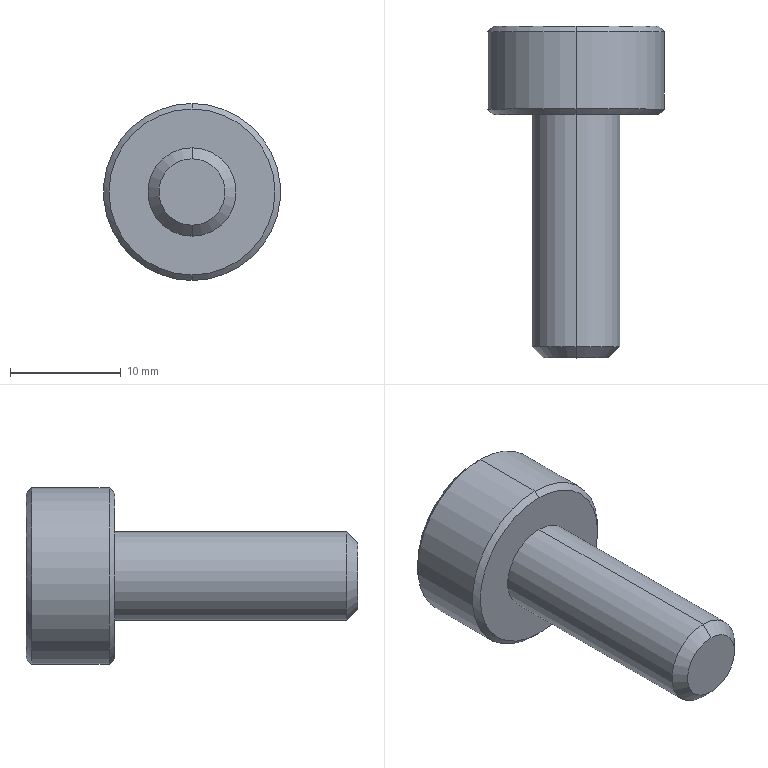Part | STEP file | Guide wheel mechanism revised.sldasm-Part-320 | 1 solid | 20 faces | box 16 x 30 x 16 mm | volume 2413 mm3 | plane 10 | cone 6 | cylinder 4 | commonest cylinder face diameters 8 x2 16 x2
STEP:
#1=CARTESIAN_POINT('',(0.,0.,-3.));
#2=VERTEX_POINT('',#1);
#3=CARTESIAN_POINT('',(0.,0.,3.));
#4=VERTEX_POINT('',#3);
#5=CARTESIAN_POINT('',(0.,0.,0.));
#6=DIRECTION('',(0.,-1.,0.));
#7=DIRECTION('',(0.,0.,-1.));
#8=AXIS2_PLACEMENT_3D('',#5,#6,#7);
#9=CIRCLE('',#8,3.);
#10=EDGE_CURVE('',#2,#4,#9,.T.);
#11=ORIENTED_EDGE('',*,*,#10,.F.);
#12=CARTESIAN_POINT('',(0.,1.,-4.));
#13=VERTEX_POINT('',#12);
#14=CARTESIAN_POINT('',(0.,0.,-3.));
#15=DIRECTION('',(0.,0.7071,-0.7071));
#16=VECTOR('',#15,1000.);
#17=LINE('',#14,#16);
#18=EDGE_CURVE('',#2,#13,#17,.T.);
#19=ORIENTED_EDGE('',*,*,#18,.T.);
#20=CARTESIAN_POINT('',(0.,1.,4.));
#21=VERTEX_POINT('',#20);
#22=CARTESIAN_POINT('',(0.,1.,0.));
#23=DIRECTION('',(0.,1.,0.));
#24=DIRECTION('',(0.,0.,-1.));
#25=AXIS2_PLACEMENT_3D('',#22,#23,#24);
#26=CIRCLE('',#25,4.);
#27=EDGE_CURVE('',#21,#13,#26,.T.);
#28=ORIENTED_EDGE('',*,*,#27,.F.);
#29=CARTESIAN_POINT('',(0.,0.,3.));
#30=DIRECTION('',(0.,0.7071,0.7071));
#31=VECTOR('',#30,1000.);
#32=LINE('',#29,#31);
#33=EDGE_CURVE('',#4,#21,#32,.T.);
#34=ORIENTED_EDGE('',*,*,#33,.F.);
#35=EDGE_LOOP('',(#11,#19,#28,#34));
#36=FACE_OUTER_BOUND('',#35,.T.);
#37=CARTESIAN_POINT('',(0.,0.,0.));
#38=DIRECTION('',(0.,1.,0.));
#39=DIRECTION('',(0.,0.,1.));
#40=AXIS2_PLACEMENT_3D('',#37,#38,#39);
#41=CONICAL_SURFACE('',#40,3.,0.7854);
#42=ADVANCED_FACE('',(#36),#41,.T.);
#43=CARTESIAN_POINT('',(0.,22.,-7.5));
#44=VERTEX_POINT('',#43);
#45=CARTESIAN_POINT('',(0.,22.,7.5));
#46=VERTEX_POINT('',#45);
#47=CARTESIAN_POINT('',(0.,22.,0.));
#48=DIRECTION('',(0.,-1.,0.));
#49=DIRECTION('',(0.,0.,-1.));
#50=AXIS2_PLACEMENT_3D('',#47,#48,#49);
#51=CIRCLE('',#50,7.5);
#52=EDGE_CURVE('',#44,#46,#51,.T.);
#53=ORIENTED_EDGE('',*,*,#52,.F.);
#54=CARTESIAN_POINT('',(0.,22.5,-8.));
#55=VERTEX_POINT('',#54);
#56=CARTESIAN_POINT('',(0.,22.,-7.5));
#57=DIRECTION('',(0.,0.7071,-0.7071));
#58=VECTOR('',#57,1000.);
#59=LINE('',#56,#58);
#60=EDGE_CURVE('',#44,#55,#59,.T.);
#61=ORIENTED_EDGE('',*,*,#60,.T.);
#62=CARTESIAN_POINT('',(0.,22.5,8.));
#63=VERTEX_POINT('',#62);
#64=CARTESIAN_POINT('',(0.,22.5,0.));
#65=DIRECTION('',(0.,1.,0.));
#66=DIRECTION('',(0.,0.,-1.));
#67=AXIS2_PLACEMENT_3D('',#64,#65,#66);
#68=CIRCLE('',#67,8.);
#69=EDGE_CURVE('',#63,#55,#68,.T.);
#70=ORIENTED_EDGE('',*,*,#69,.F.);
#71=CARTESIAN_POINT('',(0.,22.,7.5));
#72=DIRECTION('',(0.,0.7071,0.7071));
#73=VECTOR('',#72,1000.);
#74=LINE('',#71,#73);
#75=EDGE_CURVE('',#46,#63,#74,.T.);
#76=ORIENTED_EDGE('',*,*,#75,.F.);
#77=EDGE_LOOP('',(#53,#61,#70,#76));
#78=FACE_OUTER_BOUND('',#77,.T.);
#79=CARTESIAN_POINT('',(0.,22.,0.));
#80=DIRECTION('',(0.,1.,0.));
#81=DIRECTION('',(0.,0.,1.));
#82=AXIS2_PLACEMENT_3D('',#79,#80,#81);
#83=CONICAL_SURFACE('',#82,7.5,0.7854);
#84=ADVANCED_FACE('',(#78),#83,.T.);
#85=CARTESIAN_POINT('',(0.,30.,7.5));
#86=VERTEX_POINT('',#85);
#87=CARTESIAN_POINT('',(0.,30.,-7.5));
#88=VERTEX_POINT('',#87);
#89=CARTESIAN_POINT('',(0.,30.,0.));
#90=DIRECTION('',(0.,1.,0.));
#91=DIRECTION('',(0.,0.,1.));
#92=AXIS2_PLACEMENT_3D('',#89,#90,#91);
#93=CIRCLE('',#92,7.5);
#94=EDGE_CURVE('',#86,#88,#93,.T.);
#95=ORIENTED_EDGE('',*,*,#94,.F.);
#96=CARTESIAN_POINT('',(0.,29.5,8.));
#97=VERTEX_POINT('',#96);
#98=CARTESIAN_POINT('',(0.,29.5,8.));
#99=DIRECTION('',(0.,-0.7071,0.7071));
#100=VECTOR('',#99,1000.);
#101=LINE('',#98,#100);
#102=EDGE_CURVE('',#86,#97,#101,.T.);
#103=ORIENTED_EDGE('',*,*,#102,.T.);
#104=CARTESIAN_POINT('',(0.,29.5,-8.));
#105=VERTEX_POINT('',#104);
#106=CARTESIAN_POINT('',(0.,29.5,0.));
#107=DIRECTION('',(0.,-1.,0.));
#108=DIRECTION('',(0.,0.,1.));
#109=AXIS2_PLACEMENT_3D('',#106,#107,#108);
#110=CIRCLE('',#109,8.);
#111=EDGE_CURVE('',#105,#97,#110,.T.);
#112=ORIENTED_EDGE('',*,*,#111,.F.);
#113=CARTESIAN_POINT('',(0.,29.5,-8.));
#114=DIRECTION('',(0.,-0.7071,-0.7071));
#115=VECTOR('',#114,1000.);
#116=LINE('',#113,#115);
#117=EDGE_CURVE('',#88,#105,#116,.T.);
#118=ORIENTED_EDGE('',*,*,#117,.F.);
#119=EDGE_LOOP('',(#95,#103,#112,#118));
#120=FACE_OUTER_BOUND('',#119,.T.);
#121=CARTESIAN_POINT('',(0.,29.5,0.));
#122=DIRECTION('',(0.,-1.,0.));
#123=DIRECTION('',(0.,0.,-1.));
#124=AXIS2_PLACEMENT_3D('',#121,#122,#123);
#125=CONICAL_SURFACE('',#124,8.,0.7854);
#126=ADVANCED_FACE('',(#120),#125,.T.);
#127=CARTESIAN_POINT('',(0.,22.,-4.));
#128=VERTEX_POINT('',#127);
#129=CARTESIAN_POINT('',(0.,22.,4.));
#130=VERTEX_POINT('',#129);
#131=CARTESIAN_POINT('',(0.,22.,0.));
#132=DIRECTION('',(0.,-1.,0.));
#133=DIRECTION('',(0.,0.,-1.));
#134=AXIS2_PLACEMENT_3D('',#131,#132,#133);
#135=CIRCLE('',#134,4.);
#136=EDGE_CURVE('',#128,#130,#135,.T.);
#137=ORIENTED_EDGE('',*,*,#136,.T.);
#138=CARTESIAN_POINT('',(0.,0.,4.));
#139=DIRECTION('',(0.,-1.,0.));
#140=VECTOR('',#139,1000.);
#141=LINE('',#138,#140);
#142=EDGE_CURVE('',#130,#21,#141,.T.);
#143=ORIENTED_EDGE('',*,*,#142,.T.);
#144=ORIENTED_EDGE('',*,*,#27,.T.);
#145=CARTESIAN_POINT('',(0.,0.,-4.));
#146=DIRECTION('',(0.,-1.,0.));
#147=VECTOR('',#146,1000.);
#148=LINE('',#145,#147);
#149=EDGE_CURVE('',#128,#13,#148,.T.);
#150=ORIENTED_EDGE('',*,*,#149,.F.);
#151=EDGE_LOOP('',(#137,#143,#144,#150));
#152=FACE_OUTER_BOUND('',#151,.T.);
#153=CARTESIAN_POINT('',(0.,0.,0.));
#154=DIRECTION('',(0.,-1.,0.));
#155=DIRECTION('',(0.,0.,-1.));
#156=AXIS2_PLACEMENT_3D('',#153,#154,#155);
#157=CYLINDRICAL_SURFACE('',#156,4.);
#158=ADVANCED_FACE('',(#152),#157,.T.);
#159=ORIENTED_EDGE('',*,*,#111,.T.);
#160=CARTESIAN_POINT('',(0.,0.,8.));
#161=DIRECTION('',(0.,-1.,0.));
#162=VECTOR('',#161,1000.);
#163=LINE('',#160,#162);
#164=EDGE_CURVE('',#97,#63,#163,.T.);
#165=ORIENTED_EDGE('',*,*,#164,.T.);
#166=ORIENTED_EDGE('',*,*,#69,.T.);
#167=CARTESIAN_POINT('',(0.,0.,-8.));
#168=DIRECTION('',(0.,-1.,0.));
#169=VECTOR('',#168,1000.);
#170=LINE('',#167,#169);
#171=EDGE_CURVE('',#105,#55,#170,.T.);
#172=ORIENTED_EDGE('',*,*,#171,.F.);
#173=EDGE_LOOP('',(#159,#165,#166,#172));
#174=FACE_OUTER_BOUND('',#173,.T.);
#175=CARTESIAN_POINT('',(0.,0.,0.));
#176=DIRECTION('',(0.,-1.,0.));
#177=DIRECTION('',(0.,0.,-1.));
#178=AXIS2_PLACEMENT_3D('',#175,#176,#177);
#179=CYLINDRICAL_SURFACE('',#178,8.);
#180=ADVANCED_FACE('',(#174),#179,.T.);
#181=CARTESIAN_POINT('',(0.,0.,0.));
#182=DIRECTION('',(0.,-1.,0.));
#183=DIRECTION('',(0.,0.,-1.));
#184=AXIS2_PLACEMENT_3D('',#181,#182,#183);
#185=CIRCLE('',#184,3.);
#186=EDGE_CURVE('',#4,#2,#185,.T.);
#187=ORIENTED_EDGE('',*,*,#186,.T.);
#188=ORIENTED_EDGE('',*,*,#10,.T.);
#189=EDGE_LOOP('',(#187,#188));
#190=FACE_OUTER_BOUND('',#189,.T.);
#191=CARTESIAN_POINT('',(4.,0.,0.));
#192=DIRECTION('',(0.,-1.,0.));
#193=DIRECTION('',(0.,0.,-1.));
#194=AXIS2_PLACEMENT_3D('',#191,#192,#193);
#195=PLANE('',#194);
#196=ADVANCED_FACE('',(#190),#195,.T.);
#197=CARTESIAN_POINT('',(0.,30.,0.));
#198=DIRECTION('',(0.,1.,0.));
#199=DIRECTION('',(0.,0.,1.));
#200=AXIS2_PLACEMENT_3D('',#197,#198,#199);
#201=CIRCLE('',#200,7.5);
#202=EDGE_CURVE('',#88,#86,#201,.T.);
#203=ORIENTED_EDGE('',*,*,#202,.T.);
#204=ORIENTED_EDGE('',*,*,#94,.T.);
#205=EDGE_LOOP('',(#203,#204));
#206=FACE_OUTER_BOUND('',#205,.T.);
#207=CARTESIAN_POINT('',(4.,30.,-2.309));
#208=VERTEX_POINT('',#207);
#209=CARTESIAN_POINT('',(0.,30.,-4.619));
#210=VERTEX_POINT('',#209);
#211=CARTESIAN_POINT('',(4.,30.,-2.309));
#212=DIRECTION('',(-0.866,0.,-0.5));
#213=VECTOR('',#212,1000.);
#214=LINE('',#211,#213);
#215=EDGE_CURVE('',#208,#210,#214,.T.);
#216=ORIENTED_EDGE('',*,*,#215,.F.);
#217=CARTESIAN_POINT('',(4.,30.,2.309));
#218=VERTEX_POINT('',#217);
#219=CARTESIAN_POINT('',(4.,30.,2.309));
#220=DIRECTION('',(0.,0.,-1.));
#221=VECTOR('',#220,1000.);
#222=LINE('',#219,#221);
#223=EDGE_CURVE('',#218,#208,#222,.T.);
#224=ORIENTED_EDGE('',*,*,#223,.F.);
#225=CARTESIAN_POINT('',(0.,30.,4.619));
#226=VERTEX_POINT('',#225);
#227=CARTESIAN_POINT('',(0.,30.,4.619));
#228=DIRECTION('',(0.866,0.,-0.5));
#229=VECTOR('',#228,1000.);
#230=LINE('',#227,#229);
#231=EDGE_CURVE('',#226,#218,#230,.T.);
#232=ORIENTED_EDGE('',*,*,#231,.F.);
#233=CARTESIAN_POINT('',(-4.,30.,2.309));
#234=VERTEX_POINT('',#233);
#235=CARTESIAN_POINT('',(-4.,30.,2.309));
#236=DIRECTION('',(0.866,0.,0.5));
#237=VECTOR('',#236,1000.);
#238=LINE('',#235,#237);
#239=EDGE_CURVE('',#234,#226,#238,.T.);
#240=ORIENTED_EDGE('',*,*,#239,.F.);
#241=CARTESIAN_POINT('',(-4.,30.,-2.309));
#242=VERTEX_POINT('',#241);
#243=CARTESIAN_POINT('',(-4.,30.,-2.309));
#244=DIRECTION('',(0.,0.,1.));
#245=VECTOR('',#244,1000.);
#246=LINE('',#243,#245);
#247=EDGE_CURVE('',#242,#234,#246,.T.);
#248=ORIENTED_EDGE('',*,*,#247,.F.);
#249=CARTESIAN_POINT('',(0.,30.,-4.619));
#250=DIRECTION('',(-0.866,0.,0.5));
#251=VECTOR('',#250,1000.);
#252=LINE('',#249,#251);
#253=EDGE_CURVE('',#210,#242,#252,.T.);
#254=ORIENTED_EDGE('',*,*,#253,.F.);
#255=EDGE_LOOP('',(#216,#224,#232,#240,#248,#254));
#256=FACE_BOUND('',#255,.T.);
#257=CARTESIAN_POINT('',(0.,30.,0.));
#258=DIRECTION('',(0.,1.,0.));
#259=DIRECTION('',(0.,0.,1.));
#260=AXIS2_PLACEMENT_3D('',#257,#258,#259);
#261=PLANE('',#260);
#262=ADVANCED_FACE('',(#206,#256),#261,.T.);
#263=ORIENTED_EDGE('',*,*,#164,.F.);
#264=CARTESIAN_POINT('',(0.,29.5,0.));
#265=DIRECTION('',(0.,-1.,0.));
#266=DIRECTION('',(0.,0.,1.));
#267=AXIS2_PLACEMENT_3D('',#264,#265,#266);
#268=CIRCLE('',#267,8.);
#269=EDGE_CURVE('',#97,#105,#268,.T.);
#270=ORIENTED_EDGE('',*,*,#269,.T.);
#271=ORIENTED_EDGE('',*,*,#171,.T.);
#272=CARTESIAN_POINT('',(0.,22.5,0.));
#273=DIRECTION('',(0.,1.,0.));
#274=DIRECTION('',(0.,0.,-1.));
#275=AXIS2_PLACEMENT_3D('',#272,#273,#274);
#276=CIRCLE('',#275,8.);
#277=EDGE_CURVE('',#55,#63,#276,.T.);
#278=ORIENTED_EDGE('',*,*,#277,.T.);
#279=EDGE_LOOP('',(#263,#270,#271,#278));
#280=FACE_OUTER_BOUND('',#279,.T.);
#281=CARTESIAN_POINT('',(0.,0.,0.));
#282=DIRECTION('',(0.,-1.,0.));
#283=DIRECTION('',(0.,0.,-1.));
#284=AXIS2_PLACEMENT_3D('',#281,#282,#283);
#285=CYLINDRICAL_SURFACE('',#284,8.);
#286=ADVANCED_FACE('',(#280),#285,.T.);
#287=CARTESIAN_POINT('',(0.,22.,0.));
#288=DIRECTION('',(0.,-1.,0.));
#289=DIRECTION('',(0.,0.,-1.));
#290=AXIS2_PLACEMENT_3D('',#287,#288,#289);
#291=CIRCLE('',#290,7.5);
#292=EDGE_CURVE('',#46,#44,#291,.T.);
#293=ORIENTED_EDGE('',*,*,#292,.T.);
#294=ORIENTED_EDGE('',*,*,#52,.T.);
#295=EDGE_LOOP('',(#293,#294));
#296=FACE_OUTER_BOUND('',#295,.T.);
#297=ORIENTED_EDGE('',*,*,#136,.F.);
#298=CARTESIAN_POINT('',(0.,22.,0.));
#299=DIRECTION('',(0.,-1.,0.));
#300=DIRECTION('',(0.,0.,-1.));
#301=AXIS2_PLACEMENT_3D('',#298,#299,#300);
#302=CIRCLE('',#301,4.);
#303=EDGE_CURVE('',#130,#128,#302,.T.);
#304=ORIENTED_EDGE('',*,*,#303,.F.);
#305=EDGE_LOOP('',(#297,#304));
#306=FACE_BOUND('',#305,.T.);
#307=CARTESIAN_POINT('',(8.,22.,0.));
#308=DIRECTION('',(0.,-1.,0.));
#309=DIRECTION('',(0.,0.,-1.));
#310=AXIS2_PLACEMENT_3D('',#307,#308,#309);
#311=PLANE('',#310);
#312=ADVANCED_FACE('',(#296,#306),#311,.T.);
#313=ORIENTED_EDGE('',*,*,#142,.F.);
#314=ORIENTED_EDGE('',*,*,#303,.T.);
#315=ORIENTED_EDGE('',*,*,#149,.T.);
#316=CARTESIAN_POINT('',(0.,1.,0.));
#317=DIRECTION('',(0.,1.,0.));
#318=DIRECTION('',(0.,0.,-1.));
#319=AXIS2_PLACEMENT_3D('',#316,#317,#318);
#320=CIRCLE('',#319,4.);
#321=EDGE_CURVE('',#13,#21,#320,.T.);
#322=ORIENTED_EDGE('',*,*,#321,.T.);
#323=EDGE_LOOP('',(#313,#314,#315,#322));
#324=FACE_OUTER_BOUND('',#323,.T.);
#325=CARTESIAN_POINT('',(0.,0.,0.));
#326=DIRECTION('',(0.,-1.,0.));
#327=DIRECTION('',(0.,0.,-1.));
#328=AXIS2_PLACEMENT_3D('',#325,#326,#327);
#329=CYLINDRICAL_SURFACE('',#328,4.);
#330=ADVANCED_FACE('',(#324),#329,.T.);
#331=ORIENTED_EDGE('',*,*,#215,.T.);
#332=CARTESIAN_POINT('',(0.,25.,-4.619));
#333=VERTEX_POINT('',#332);
#334=CARTESIAN_POINT('',(0.,25.,-4.619));
#335=DIRECTION('',(0.,1.,0.));
#336=VECTOR('',#335,1000.);
#337=LINE('',#334,#336);
#338=EDGE_CURVE('',#333,#210,#337,.T.);
#339=ORIENTED_EDGE('',*,*,#338,.F.);
#340=CARTESIAN_POINT('',(4.,25.,-2.309));
#341=VERTEX_POINT('',#340);
#342=CARTESIAN_POINT('',(4.,25.,-2.309));
#343=DIRECTION('',(-0.866,0.,-0.5));
#344=VECTOR('',#343,1000.);
#345=LINE('',#342,#344);
#346=EDGE_CURVE('',#341,#333,#345,.T.);
#347=ORIENTED_EDGE('',*,*,#346,.F.);
#348=CARTESIAN_POINT('',(4.,25.,-2.309));
#349=DIRECTION('',(0.,1.,0.));
#350=VECTOR('',#349,1000.);
#351=LINE('',#348,#350);
#352=EDGE_CURVE('',#341,#208,#351,.T.);
#353=ORIENTED_EDGE('',*,*,#352,.T.);
#354=EDGE_LOOP('',(#331,#339,#347,#353));
#355=FACE_OUTER_BOUND('',#354,.T.);
#356=CARTESIAN_POINT('',(4.,25.,-2.309));
#357=DIRECTION('',(0.5,0.,-0.866));
#358=DIRECTION('',(-0.866,0.,-0.5));
#359=AXIS2_PLACEMENT_3D('',#356,#357,#358);
#360=PLANE('',#359);
#361=ADVANCED_FACE('',(#355),#360,.F.);
#362=ORIENTED_EDGE('',*,*,#223,.T.);
#363=ORIENTED_EDGE('',*,*,#352,.F.);
#364=CARTESIAN_POINT('',(4.,25.,2.309));
#365=VERTEX_POINT('',#364);
#366=CARTESIAN_POINT('',(4.,25.,2.309));
#367=DIRECTION('',(0.,0.,-1.));
#368=VECTOR('',#367,1000.);
#369=LINE('',#366,#368);
#370=EDGE_CURVE('',#365,#341,#369,.T.);
#371=ORIENTED_EDGE('',*,*,#370,.F.);
#372=CARTESIAN_POINT('',(4.,25.,2.309));
#373=DIRECTION('',(0.,1.,0.));
#374=VECTOR('',#373,1000.);
#375=LINE('',#372,#374);
#376=EDGE_CURVE('',#365,#218,#375,.T.);
#377=ORIENTED_EDGE('',*,*,#376,.T.);
#378=EDGE_LOOP('',(#362,#363,#371,#377));
#379=FACE_OUTER_BOUND('',#378,.T.);
#380=CARTESIAN_POINT('',(4.,25.,2.309));
#381=DIRECTION('',(1.,0.,0.));
#382=DIRECTION('',(0.,0.,-1.));
#383=AXIS2_PLACEMENT_3D('',#380,#381,#382);
#384=PLANE('',#383);
#385=ADVANCED_FACE('',(#379),#384,.F.);
#386=ORIENTED_EDGE('',*,*,#231,.T.);
#387=ORIENTED_EDGE('',*,*,#376,.F.);
#388=CARTESIAN_POINT('',(0.,25.,4.619));
#389=VERTEX_POINT('',#388);
#390=CARTESIAN_POINT('',(0.,25.,4.619));
#391=DIRECTION('',(0.866,0.,-0.5));
#392=VECTOR('',#391,1000.);
#393=LINE('',#390,#392);
#394=EDGE_CURVE('',#389,#365,#393,.T.);
#395=ORIENTED_EDGE('',*,*,#394,.F.);
#396=CARTESIAN_POINT('',(0.,25.,4.619));
#397=DIRECTION('',(0.,1.,0.));
#398=VECTOR('',#397,1000.);
#399=LINE('',#396,#398);
#400=EDGE_CURVE('',#389,#226,#399,.T.);
#401=ORIENTED_EDGE('',*,*,#400,.T.);
#402=EDGE_LOOP('',(#386,#387,#395,#401));
#403=FACE_OUTER_BOUND('',#402,.T.);
#404=CARTESIAN_POINT('',(0.,25.,4.619));
#405=DIRECTION('',(0.5,0.,0.866));
#406=DIRECTION('',(0.866,0.,-0.5));
#407=AXIS2_PLACEMENT_3D('',#404,#405,#406);
#408=PLANE('',#407);
#409=ADVANCED_FACE('',(#403),#408,.F.);
#410=ORIENTED_EDGE('',*,*,#239,.T.);
#411=ORIENTED_EDGE('',*,*,#400,.F.);
#412=CARTESIAN_POINT('',(-4.,25.,2.309));
#413=VERTEX_POINT('',#412);
#414=CARTESIAN_POINT('',(-4.,25.,2.309));
#415=DIRECTION('',(0.866,0.,0.5));
#416=VECTOR('',#415,1000.);
#417=LINE('',#414,#416);
#418=EDGE_CURVE('',#413,#389,#417,.T.);
#419=ORIENTED_EDGE('',*,*,#418,.F.);
#420=CARTESIAN_POINT('',(-4.,25.,2.309));
#421=DIRECTION('',(0.,1.,0.));
#422=VECTOR('',#421,1000.);
#423=LINE('',#420,#422);
#424=EDGE_CURVE('',#413,#234,#423,.T.);
#425=ORIENTED_EDGE('',*,*,#424,.T.);
#426=EDGE_LOOP('',(#410,#411,#419,#425));
#427=FACE_OUTER_BOUND('',#426,.T.);
#428=CARTESIAN_POINT('',(-4.,25.,2.309));
#429=DIRECTION('',(-0.5,0.,0.866));
#430=DIRECTION('',(0.866,0.,0.5));
#431=AXIS2_PLACEMENT_3D('',#428,#429,#430);
#432=PLANE('',#431);
#433=ADVANCED_FACE('',(#427),#432,.F.);
#434=ORIENTED_EDGE('',*,*,#247,.T.);
#435=ORIENTED_EDGE('',*,*,#424,.F.);
#436=CARTESIAN_POINT('',(-4.,25.,-2.309));
#437=VERTEX_POINT('',#436);
#438=CARTESIAN_POINT('',(-4.,25.,-2.309));
#439=DIRECTION('',(0.,0.,1.));
#440=VECTOR('',#439,1000.);
#441=LINE('',#438,#440);
#442=EDGE_CURVE('',#437,#413,#441,.T.);
#443=ORIENTED_EDGE('',*,*,#442,.F.);
#444=CARTESIAN_POINT('',(-4.,25.,-2.309));
#445=DIRECTION('',(0.,1.,0.));
#446=VECTOR('',#445,1000.);
#447=LINE('',#444,#446);
#448=EDGE_CURVE('',#437,#242,#447,.T.);
#449=ORIENTED_EDGE('',*,*,#448,.T.);
#450=EDGE_LOOP('',(#434,#435,#443,#449));
#451=FACE_OUTER_BOUND('',#450,.T.);
#452=CARTESIAN_POINT('',(-4.,25.,-2.309));
#453=DIRECTION('',(-1.,0.,0.));
#454=DIRECTION('',(0.,0.,1.));
#455=AXIS2_PLACEMENT_3D('',#452,#453,#454);
#456=PLANE('',#455);
#457=ADVANCED_FACE('',(#451),#456,.F.);
#458=ORIENTED_EDGE('',*,*,#253,.T.);
#459=ORIENTED_EDGE('',*,*,#448,.F.);
#460=CARTESIAN_POINT('',(0.,25.,-4.619));
#461=DIRECTION('',(-0.866,0.,0.5));
#462=VECTOR('',#461,1000.);
#463=LINE('',#460,#462);
#464=EDGE_CURVE('',#333,#437,#463,.T.);
#465=ORIENTED_EDGE('',*,*,#464,.F.);
#466=ORIENTED_EDGE('',*,*,#338,.T.);
#467=EDGE_LOOP('',(#458,#459,#465,#466));
#468=FACE_OUTER_BOUND('',#467,.T.);
#469=CARTESIAN_POINT('',(0.,25.,-4.619));
#470=DIRECTION('',(-0.5,0.,-0.866));
#471=DIRECTION('',(-0.866,0.,0.5));
#472=AXIS2_PLACEMENT_3D('',#469,#470,#471);
#473=PLANE('',#472);
#474=ADVANCED_FACE('',(#468),#473,.F.);
#475=ORIENTED_EDGE('',*,*,#346,.T.);
#476=ORIENTED_EDGE('',*,*,#464,.T.);
#477=ORIENTED_EDGE('',*,*,#442,.T.);
#478=ORIENTED_EDGE('',*,*,#418,.T.);
#479=ORIENTED_EDGE('',*,*,#394,.T.);
#480=ORIENTED_EDGE('',*,*,#370,.T.);
#481=EDGE_LOOP('',(#475,#476,#477,#478,#479,#480));
#482=FACE_OUTER_BOUND('',#481,.T.);
#483=CARTESIAN_POINT('',(0.,25.,0.));
#484=DIRECTION('',(0.,1.,0.));
#485=DIRECTION('',(0.,0.,1.));
#486=AXIS2_PLACEMENT_3D('',#483,#484,#485);
#487=PLANE('',#486);
#488=ADVANCED_FACE('',(#482),#487,.T.);
#489=ORIENTED_EDGE('',*,*,#102,.F.);
#490=ORIENTED_EDGE('',*,*,#202,.F.);
#491=ORIENTED_EDGE('',*,*,#117,.T.);
#492=ORIENTED_EDGE('',*,*,#269,.F.);
#493=EDGE_LOOP('',(#489,#490,#491,#492));
#494=FACE_OUTER_BOUND('',#493,.T.);
#495=CARTESIAN_POINT('',(0.,29.5,0.));
#496=DIRECTION('',(0.,-1.,0.));
#497=DIRECTION('',(0.,0.,-1.));
#498=AXIS2_PLACEMENT_3D('',#495,#496,#497);
#499=CONICAL_SURFACE('',#498,8.,0.7854);
#500=ADVANCED_FACE('',(#494),#499,.T.);
#501=ORIENTED_EDGE('',*,*,#60,.F.);
#502=ORIENTED_EDGE('',*,*,#292,.F.);
#503=ORIENTED_EDGE('',*,*,#75,.T.);
#504=ORIENTED_EDGE('',*,*,#277,.F.);
#505=EDGE_LOOP('',(#501,#502,#503,#504));
#506=FACE_OUTER_BOUND('',#505,.T.);
#507=CARTESIAN_POINT('',(0.,22.,0.));
#508=DIRECTION('',(0.,1.,0.));
#509=DIRECTION('',(0.,0.,1.));
#510=AXIS2_PLACEMENT_3D('',#507,#508,#509);
#511=CONICAL_SURFACE('',#510,7.5,0.7854);
#512=ADVANCED_FACE('',(#506),#511,.T.);
#513=ORIENTED_EDGE('',*,*,#18,.F.);
#514=ORIENTED_EDGE('',*,*,#186,.F.);
#515=ORIENTED_EDGE('',*,*,#33,.T.);
#516=ORIENTED_EDGE('',*,*,#321,.F.);
#517=EDGE_LOOP('',(#513,#514,#515,#516));
#518=FACE_OUTER_BOUND('',#517,.T.);
#519=CARTESIAN_POINT('',(0.,0.,0.));
#520=DIRECTION('',(0.,1.,0.));
#521=DIRECTION('',(0.,0.,1.));
#522=AXIS2_PLACEMENT_3D('',#519,#520,#521);
#523=CONICAL_SURFACE('',#522,3.,0.7854);
#524=ADVANCED_FACE('',(#518),#523,.T.);
#525=CLOSED_SHELL('',(#42,#84,#126,#158,#180,#196,#262,#286,#312,#330,#361,#385,#409,#433,#457,#474,#488,#500,#512,#524));
#526=MANIFOLD_SOLID_BREP('',#525);
#527=CARTESIAN_POINT('',(0.,0.,0.));
#528=DIRECTION('',(0.,0.,1.));
#529=DIRECTION('',(1.,0.,0.));
#530=AXIS2_PLACEMENT_3D('',#527,#528,#529);
#531=(LENGTH_UNIT()NAMED_UNIT(*)SI_UNIT(.MILLI.,.METRE.));
#532=UNCERTAINTY_MEASURE_WITH_UNIT(LENGTH_MEASURE(0.00001),#531,'','');
#533=(NAMED_UNIT(*)PLANE_ANGLE_UNIT()SI_UNIT($,.RADIAN.));
#534=(NAMED_UNIT(*)SI_UNIT($,.STERADIAN.)SOLID_ANGLE_UNIT());
#535=(GEOMETRIC_REPRESENTATION_CONTEXT(3)GLOBAL_UNCERTAINTY_ASSIGNED_CONTEXT((#532))GLOBAL_UNIT_ASSIGNED_CONTEXT((#531,#533,#534))REPRESENTATION_CONTEXT('',''));
#536=ADVANCED_BREP_SHAPE_REPRESENTATION('',(#526,#530),#535);